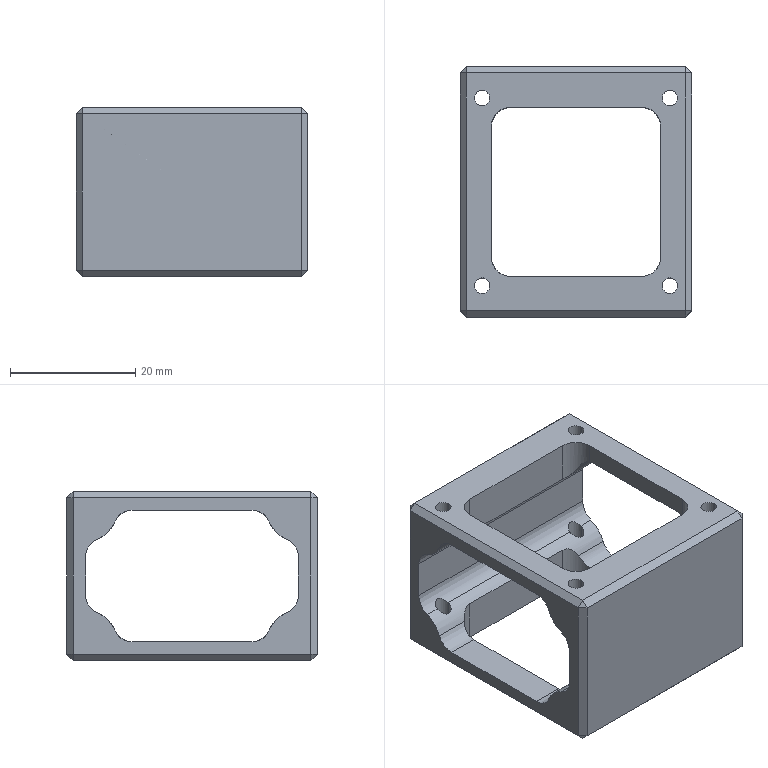Part | SolidWorks | features ICE 3, 3DProfileFeature 1, Chamfer 1, Extrusion 1, HoleWzd 1 | 1 solid | 80 faces | box 37 x 40 x 27 mm | volume 11447 mm3 | cylinder 40 | plane 40 | commonest cylinder face diameters 6 x20 2.5 x16 10 x4